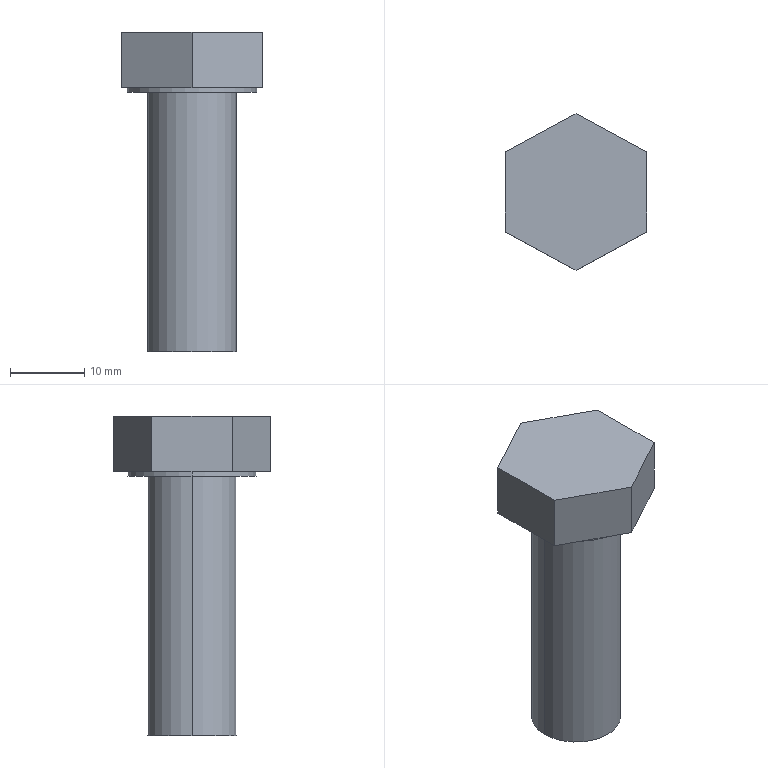Part | STEP file | M12-35 | 1 solid | 14 faces | box 19 x 21.1 x 43.1 mm | volume 6374 mm3 | plane 10 | cylinder 4 | commonest cylinder face diameters 12 x2 17.4 x2
STEP:
#1=CARTESIAN_POINT('',(0.,0.,0.));
#2=DIRECTION('',(0.,0.,1.));
#3=DIRECTION('',(1.,0.,0.));
#4=AXIS2_PLACEMENT_3D('',#1,#2,#3);
#5=CARTESIAN_POINT('',(0.,10.55,0.));
#6=VERTEX_POINT('',#5);
#7=CARTESIAN_POINT('',(-9.5,5.402,0.));
#8=VERTEX_POINT('',#7);
#9=CARTESIAN_POINT('',(0.,10.55,0.));
#10=DIRECTION('',(-0.8792,-0.4764,0.));
#11=VECTOR('',#10,1.);
#12=LINE('',#9,#11);
#13=CARTESIAN_POINT('',(0.,0.,0.));
#14=DIRECTION('',(0.,0.,1.));
#15=DIRECTION('',(1.,0.,0.));
#16=AXIS2_PLACEMENT_3D('',#13,#14,#15);
#17=PLANE('',#16);
#18=CARTESIAN_POINT('',(0.,10.55));
#19=DIRECTION('',(-0.8792,-0.4764));
#20=VECTOR('',#19,1.);
#21=LINE('',#18,#20);
#22=(GEOMETRIC_REPRESENTATION_CONTEXT(2)PARAMETRIC_REPRESENTATION_CONTEXT()REPRESENTATION_CONTEXT('',''));
#23=DEFINITIONAL_REPRESENTATION('',(#21),#22);
#24=PCURVE('',#17,#23);
#25=CARTESIAN_POINT('',(0.,10.55,0.));
#26=DIRECTION('',(-0.4764,0.8792,0.));
#27=DIRECTION('',(-0.8792,-0.4764,0.));
#28=AXIS2_PLACEMENT_3D('',#25,#26,#27);
#29=PLANE('',#28);
#30=CARTESIAN_POINT('',(0.,0.));
#31=DIRECTION('',(1.,0.));
#32=VECTOR('',#31,1.);
#33=LINE('',#30,#32);
#34=(GEOMETRIC_REPRESENTATION_CONTEXT(2)PARAMETRIC_REPRESENTATION_CONTEXT()REPRESENTATION_CONTEXT('',''));
#35=DEFINITIONAL_REPRESENTATION('',(#33),#34);
#36=PCURVE('',#29,#35);
#37=SURFACE_CURVE('',#12,(#24,#36),.PCURVE_S1.);
#38=EDGE_CURVE('',#6,#8,#37,.T.);
#39=ORIENTED_EDGE('',*,*,#38,.T.);
#40=CARTESIAN_POINT('',(-9.5,-5.402,0.));
#41=VERTEX_POINT('',#40);
#42=CARTESIAN_POINT('',(-9.5,5.402,0.));
#43=DIRECTION('',(0.,-1.,0.));
#44=VECTOR('',#43,1.);
#45=LINE('',#42,#44);
#46=CARTESIAN_POINT('',(-9.5,5.402));
#47=DIRECTION('',(0.,-1.));
#48=VECTOR('',#47,1.);
#49=LINE('',#46,#48);
#50=(GEOMETRIC_REPRESENTATION_CONTEXT(2)PARAMETRIC_REPRESENTATION_CONTEXT()REPRESENTATION_CONTEXT('',''));
#51=DEFINITIONAL_REPRESENTATION('',(#49),#50);
#52=PCURVE('',#17,#51);
#53=CARTESIAN_POINT('',(-9.5,5.402,0.));
#54=DIRECTION('',(-1.,0.,0.));
#55=DIRECTION('',(0.,-1.,0.));
#56=AXIS2_PLACEMENT_3D('',#53,#54,#55);
#57=PLANE('',#56);
#58=CARTESIAN_POINT('',(0.,0.));
#59=DIRECTION('',(1.,0.));
#60=VECTOR('',#59,1.);
#61=LINE('',#58,#60);
#62=(GEOMETRIC_REPRESENTATION_CONTEXT(2)PARAMETRIC_REPRESENTATION_CONTEXT()REPRESENTATION_CONTEXT('',''));
#63=DEFINITIONAL_REPRESENTATION('',(#61),#62);
#64=PCURVE('',#57,#63);
#65=SURFACE_CURVE('',#45,(#52,#64),.PCURVE_S1.);
#66=EDGE_CURVE('',#8,#41,#65,.T.);
#67=ORIENTED_EDGE('',*,*,#66,.T.);
#68=CARTESIAN_POINT('',(0.,-10.55,0.));
#69=VERTEX_POINT('',#68);
#70=CARTESIAN_POINT('',(-9.5,-5.402,0.));
#71=DIRECTION('',(0.8792,-0.4764,0.));
#72=VECTOR('',#71,1.);
#73=LINE('',#70,#72);
#74=CARTESIAN_POINT('',(-9.5,-5.402));
#75=DIRECTION('',(0.8792,-0.4764));
#76=VECTOR('',#75,1.);
#77=LINE('',#74,#76);
#78=(GEOMETRIC_REPRESENTATION_CONTEXT(2)PARAMETRIC_REPRESENTATION_CONTEXT()REPRESENTATION_CONTEXT('',''));
#79=DEFINITIONAL_REPRESENTATION('',(#77),#78);
#80=PCURVE('',#17,#79);
#81=CARTESIAN_POINT('',(-9.5,-5.402,0.));
#82=DIRECTION('',(-0.4764,-0.8792,0.));
#83=DIRECTION('',(0.8792,-0.4764,0.));
#84=AXIS2_PLACEMENT_3D('',#81,#82,#83);
#85=PLANE('',#84);
#86=CARTESIAN_POINT('',(0.,0.));
#87=DIRECTION('',(1.,0.));
#88=VECTOR('',#87,1.);
#89=LINE('',#86,#88);
#90=(GEOMETRIC_REPRESENTATION_CONTEXT(2)PARAMETRIC_REPRESENTATION_CONTEXT()REPRESENTATION_CONTEXT('',''));
#91=DEFINITIONAL_REPRESENTATION('',(#89),#90);
#92=PCURVE('',#85,#91);
#93=SURFACE_CURVE('',#73,(#80,#92),.PCURVE_S1.);
#94=EDGE_CURVE('',#41,#69,#93,.T.);
#95=ORIENTED_EDGE('',*,*,#94,.T.);
#96=CARTESIAN_POINT('',(9.5,-5.402,0.));
#97=VERTEX_POINT('',#96);
#98=CARTESIAN_POINT('',(0.,-10.55,0.));
#99=DIRECTION('',(0.8792,0.4764,0.));
#100=VECTOR('',#99,1.);
#101=LINE('',#98,#100);
#102=CARTESIAN_POINT('',(0.,-10.55));
#103=DIRECTION('',(0.8792,0.4764));
#104=VECTOR('',#103,1.);
#105=LINE('',#102,#104);
#106=(GEOMETRIC_REPRESENTATION_CONTEXT(2)PARAMETRIC_REPRESENTATION_CONTEXT()REPRESENTATION_CONTEXT('',''));
#107=DEFINITIONAL_REPRESENTATION('',(#105),#106);
#108=PCURVE('',#17,#107);
#109=CARTESIAN_POINT('',(0.,-10.55,0.));
#110=DIRECTION('',(0.4764,-0.8792,0.));
#111=DIRECTION('',(0.8792,0.4764,0.));
#112=AXIS2_PLACEMENT_3D('',#109,#110,#111);
#113=PLANE('',#112);
#114=CARTESIAN_POINT('',(0.,0.));
#115=DIRECTION('',(1.,0.));
#116=VECTOR('',#115,1.);
#117=LINE('',#114,#116);
#118=(GEOMETRIC_REPRESENTATION_CONTEXT(2)PARAMETRIC_REPRESENTATION_CONTEXT()REPRESENTATION_CONTEXT('',''));
#119=DEFINITIONAL_REPRESENTATION('',(#117),#118);
#120=PCURVE('',#113,#119);
#121=SURFACE_CURVE('',#101,(#108,#120),.PCURVE_S1.);
#122=EDGE_CURVE('',#69,#97,#121,.T.);
#123=ORIENTED_EDGE('',*,*,#122,.T.);
#124=CARTESIAN_POINT('',(9.5,5.402,0.));
#125=VERTEX_POINT('',#124);
#126=CARTESIAN_POINT('',(9.5,-5.402,0.));
#127=DIRECTION('',(0.,1.,0.));
#128=VECTOR('',#127,1.);
#129=LINE('',#126,#128);
#130=CARTESIAN_POINT('',(9.5,-5.402));
#131=DIRECTION('',(0.,1.));
#132=VECTOR('',#131,1.);
#133=LINE('',#130,#132);
#134=(GEOMETRIC_REPRESENTATION_CONTEXT(2)PARAMETRIC_REPRESENTATION_CONTEXT()REPRESENTATION_CONTEXT('',''));
#135=DEFINITIONAL_REPRESENTATION('',(#133),#134);
#136=PCURVE('',#17,#135);
#137=CARTESIAN_POINT('',(9.5,-5.402,0.));
#138=DIRECTION('',(1.,0.,0.));
#139=DIRECTION('',(0.,1.,0.));
#140=AXIS2_PLACEMENT_3D('',#137,#138,#139);
#141=PLANE('',#140);
#142=CARTESIAN_POINT('',(0.,0.));
#143=DIRECTION('',(1.,0.));
#144=VECTOR('',#143,1.);
#145=LINE('',#142,#144);
#146=(GEOMETRIC_REPRESENTATION_CONTEXT(2)PARAMETRIC_REPRESENTATION_CONTEXT()REPRESENTATION_CONTEXT('',''));
#147=DEFINITIONAL_REPRESENTATION('',(#145),#146);
#148=PCURVE('',#141,#147);
#149=SURFACE_CURVE('',#129,(#136,#148),.PCURVE_S1.);
#150=EDGE_CURVE('',#97,#125,#149,.T.);
#151=ORIENTED_EDGE('',*,*,#150,.T.);
#152=CARTESIAN_POINT('',(9.5,5.402,0.));
#153=DIRECTION('',(-0.8792,0.4764,0.));
#154=VECTOR('',#153,1.);
#155=LINE('',#152,#154);
#156=CARTESIAN_POINT('',(9.5,5.402));
#157=DIRECTION('',(-0.8792,0.4764));
#158=VECTOR('',#157,1.);
#159=LINE('',#156,#158);
#160=(GEOMETRIC_REPRESENTATION_CONTEXT(2)PARAMETRIC_REPRESENTATION_CONTEXT()REPRESENTATION_CONTEXT('',''));
#161=DEFINITIONAL_REPRESENTATION('',(#159),#160);
#162=PCURVE('',#17,#161);
#163=CARTESIAN_POINT('',(9.5,5.402,0.));
#164=DIRECTION('',(0.4764,0.8792,0.));
#165=DIRECTION('',(-0.8792,0.4764,0.));
#166=AXIS2_PLACEMENT_3D('',#163,#164,#165);
#167=PLANE('',#166);
#168=CARTESIAN_POINT('',(0.,0.));
#169=DIRECTION('',(1.,0.));
#170=VECTOR('',#169,1.);
#171=LINE('',#168,#170);
#172=(GEOMETRIC_REPRESENTATION_CONTEXT(2)PARAMETRIC_REPRESENTATION_CONTEXT()REPRESENTATION_CONTEXT('',''));
#173=DEFINITIONAL_REPRESENTATION('',(#171),#172);
#174=PCURVE('',#167,#173);
#175=SURFACE_CURVE('',#155,(#162,#174),.PCURVE_S1.);
#176=EDGE_CURVE('',#125,#6,#175,.T.);
#177=ORIENTED_EDGE('',*,*,#176,.T.);
#178=EDGE_LOOP('',(#39,#67,#95,#123,#151,#177));
#179=FACE_BOUND('',#178,.F.);
#180=CARTESIAN_POINT('',(-8.7,0.,0.));
#181=VERTEX_POINT('',#180);
#182=CARTESIAN_POINT('',(8.7,0.,0.));
#183=VERTEX_POINT('',#182);
#184=CARTESIAN_POINT('',(0.,0.,0.));
#185=DIRECTION('',(0.,0.,-1.));
#186=DIRECTION('',(-1.,0.,0.));
#187=AXIS2_PLACEMENT_3D('',#184,#185,#186);
#188=CIRCLE('',#187,8.7);
#189=CARTESIAN_POINT('',(-8.7,0.));
#190=CARTESIAN_POINT('',(-8.7,15.069));
#191=CARTESIAN_POINT('',(4.35,7.534));
#192=CARTESIAN_POINT('',(17.4,0.));
#193=CARTESIAN_POINT('',(4.35,-7.534));
#194=CARTESIAN_POINT('',(-8.7,-15.069));
#195=CARTESIAN_POINT('',(-8.7,0.));
#196=(BOUNDED_CURVE()B_SPLINE_CURVE(2,(#189,#190,#191,#192,#193,#194,#195),.UNSPECIFIED.,.T.,.F.)B_SPLINE_CURVE_WITH_KNOTS((1,2,2,2,2,1),(-2.094,0.,2.094,4.189,6.283,8.378),.UNSPECIFIED.)CURVE()GEOMETRIC_REPRESENTATION_ITEM()RATIONAL_B_SPLINE_CURVE((1.,0.5,1.,0.5,1.,0.5,1.))REPRESENTATION_ITEM(''));
#197=(GEOMETRIC_REPRESENTATION_CONTEXT(2)PARAMETRIC_REPRESENTATION_CONTEXT()REPRESENTATION_CONTEXT('',''));
#198=DEFINITIONAL_REPRESENTATION('',(#196),#197);
#199=PCURVE('',#17,#198);
#200=CARTESIAN_POINT('',(0.,0.,0.));
#201=DIRECTION('',(0.,0.,-1.));
#202=DIRECTION('',(-1.,0.,0.));
#203=AXIS2_PLACEMENT_3D('',#200,#201,#202);
#204=CYLINDRICAL_SURFACE('',#203,8.7);
#205=CARTESIAN_POINT('',(0.,0.));
#206=DIRECTION('',(1.,0.));
#207=VECTOR('',#206,1.);
#208=LINE('',#205,#207);
#209=(GEOMETRIC_REPRESENTATION_CONTEXT(2)PARAMETRIC_REPRESENTATION_CONTEXT()REPRESENTATION_CONTEXT('',''));
#210=DEFINITIONAL_REPRESENTATION('',(#208),#209);
#211=PCURVE('',#204,#210);
#212=SURFACE_CURVE('',#188,(#199,#211),.PCURVE_S1.);
#213=EDGE_CURVE('',#181,#183,#212,.T.);
#214=ORIENTED_EDGE('',*,*,#213,.T.);
#215=CARTESIAN_POINT('',(0.,0.,0.));
#216=DIRECTION('',(0.,0.,-1.));
#217=DIRECTION('',(1.,0.,0.));
#218=AXIS2_PLACEMENT_3D('',#215,#216,#217);
#219=CIRCLE('',#218,8.7);
#220=CARTESIAN_POINT('',(8.7,0.));
#221=CARTESIAN_POINT('',(8.7,-15.069));
#222=CARTESIAN_POINT('',(-4.35,-7.534));
#223=CARTESIAN_POINT('',(-17.4,0.));
#224=CARTESIAN_POINT('',(-4.35,7.534));
#225=CARTESIAN_POINT('',(8.7,15.069));
#226=CARTESIAN_POINT('',(8.7,0.));
#227=(BOUNDED_CURVE()B_SPLINE_CURVE(2,(#220,#221,#222,#223,#224,#225,#226),.UNSPECIFIED.,.T.,.F.)B_SPLINE_CURVE_WITH_KNOTS((1,2,2,2,2,1),(-2.094,0.,2.094,4.189,6.283,8.378),.UNSPECIFIED.)CURVE()GEOMETRIC_REPRESENTATION_ITEM()RATIONAL_B_SPLINE_CURVE((1.,0.5,1.,0.5,1.,0.5,1.))REPRESENTATION_ITEM(''));
#228=(GEOMETRIC_REPRESENTATION_CONTEXT(2)PARAMETRIC_REPRESENTATION_CONTEXT()REPRESENTATION_CONTEXT('',''));
#229=DEFINITIONAL_REPRESENTATION('',(#227),#228);
#230=PCURVE('',#17,#229);
#231=CARTESIAN_POINT('',(0.,0.,0.));
#232=DIRECTION('',(0.,0.,-1.));
#233=DIRECTION('',(-1.,0.,0.));
#234=AXIS2_PLACEMENT_3D('',#231,#232,#233);
#235=CYLINDRICAL_SURFACE('',#234,8.7);
#236=CARTESIAN_POINT('',(3.142,0.));
#237=DIRECTION('',(1.,0.));
#238=VECTOR('',#237,1.);
#239=LINE('',#236,#238);
#240=(GEOMETRIC_REPRESENTATION_CONTEXT(2)PARAMETRIC_REPRESENTATION_CONTEXT()REPRESENTATION_CONTEXT('',''));
#241=DEFINITIONAL_REPRESENTATION('',(#239),#240);
#242=PCURVE('',#235,#241);
#243=SURFACE_CURVE('',#219,(#230,#242),.PCURVE_S1.);
#244=EDGE_CURVE('',#183,#181,#243,.T.);
#245=ORIENTED_EDGE('',*,*,#244,.T.);
#246=EDGE_LOOP('',(#214,#245));
#247=FACE_BOUND('',#246,.F.);
#248=ADVANCED_FACE('',(#179,#247),#17,.F.);
#249=ORIENTED_EDGE('',*,*,#38,.F.);
#250=CARTESIAN_POINT('',(0.,10.55,7.5));
#251=VERTEX_POINT('',#250);
#252=CARTESIAN_POINT('',(0.,10.55,0.));
#253=DIRECTION('',(0.,0.,1.));
#254=VECTOR('',#253,1.);
#255=LINE('',#252,#254);
#256=CARTESIAN_POINT('',(0.,0.));
#257=DIRECTION('',(0.,1.));
#258=VECTOR('',#257,1.);
#259=LINE('',#256,#258);
#260=(GEOMETRIC_REPRESENTATION_CONTEXT(2)PARAMETRIC_REPRESENTATION_CONTEXT()REPRESENTATION_CONTEXT('',''));
#261=DEFINITIONAL_REPRESENTATION('',(#259),#260);
#262=PCURVE('',#29,#261);
#263=CARTESIAN_POINT('',(10.805,0.));
#264=DIRECTION('',(0.,1.));
#265=VECTOR('',#264,1.);
#266=LINE('',#263,#265);
#267=(GEOMETRIC_REPRESENTATION_CONTEXT(2)PARAMETRIC_REPRESENTATION_CONTEXT()REPRESENTATION_CONTEXT('',''));
#268=DEFINITIONAL_REPRESENTATION('',(#266),#267);
#269=PCURVE('',#167,#268);
#270=SURFACE_CURVE('',#255,(#262,#269),.PCURVE_S1.);
#271=EDGE_CURVE('',#6,#251,#270,.T.);
#272=ORIENTED_EDGE('',*,*,#271,.T.);
#273=CARTESIAN_POINT('',(-9.5,5.402,7.5));
#274=VERTEX_POINT('',#273);
#275=CARTESIAN_POINT('',(0.,10.55,7.5));
#276=DIRECTION('',(-0.8792,-0.4764,0.));
#277=VECTOR('',#276,1.);
#278=LINE('',#275,#277);
#279=CARTESIAN_POINT('',(0.,7.5));
#280=DIRECTION('',(1.,0.));
#281=VECTOR('',#280,1.);
#282=LINE('',#279,#281);
#283=(GEOMETRIC_REPRESENTATION_CONTEXT(2)PARAMETRIC_REPRESENTATION_CONTEXT()REPRESENTATION_CONTEXT('',''));
#284=DEFINITIONAL_REPRESENTATION('',(#282),#283);
#285=PCURVE('',#29,#284);
#286=CARTESIAN_POINT('',(0.,0.,7.5));
#287=DIRECTION('',(0.,0.,1.));
#288=DIRECTION('',(1.,0.,0.));
#289=AXIS2_PLACEMENT_3D('',#286,#287,#288);
#290=PLANE('',#289);
#291=CARTESIAN_POINT('',(0.,10.55));
#292=DIRECTION('',(-0.8792,-0.4764));
#293=VECTOR('',#292,1.);
#294=LINE('',#291,#293);
#295=(GEOMETRIC_REPRESENTATION_CONTEXT(2)PARAMETRIC_REPRESENTATION_CONTEXT()REPRESENTATION_CONTEXT('',''));
#296=DEFINITIONAL_REPRESENTATION('',(#294),#295);
#297=PCURVE('',#290,#296);
#298=SURFACE_CURVE('',#278,(#285,#297),.PCURVE_S1.);
#299=EDGE_CURVE('',#251,#274,#298,.T.);
#300=ORIENTED_EDGE('',*,*,#299,.T.);
#301=CARTESIAN_POINT('',(-9.5,5.402,0.));
#302=DIRECTION('',(0.,0.,1.));
#303=VECTOR('',#302,1.);
#304=LINE('',#301,#303);
#305=CARTESIAN_POINT('',(10.805,0.));
#306=DIRECTION('',(0.,1.));
#307=VECTOR('',#306,1.);
#308=LINE('',#305,#307);
#309=(GEOMETRIC_REPRESENTATION_CONTEXT(2)PARAMETRIC_REPRESENTATION_CONTEXT()REPRESENTATION_CONTEXT('',''));
#310=DEFINITIONAL_REPRESENTATION('',(#308),#309);
#311=PCURVE('',#29,#310);
#312=CARTESIAN_POINT('',(0.,0.));
#313=DIRECTION('',(0.,1.));
#314=VECTOR('',#313,1.);
#315=LINE('',#312,#314);
#316=(GEOMETRIC_REPRESENTATION_CONTEXT(2)PARAMETRIC_REPRESENTATION_CONTEXT()REPRESENTATION_CONTEXT('',''));
#317=DEFINITIONAL_REPRESENTATION('',(#315),#316);
#318=PCURVE('',#57,#317);
#319=SURFACE_CURVE('',#304,(#311,#318),.PCURVE_S1.);
#320=EDGE_CURVE('',#8,#274,#319,.T.);
#321=ORIENTED_EDGE('',*,*,#320,.F.);
#322=EDGE_LOOP('',(#249,#272,#300,#321));
#323=FACE_BOUND('',#322,.F.);
#324=ADVANCED_FACE('',(#323),#29,.T.);
#325=ORIENTED_EDGE('',*,*,#176,.F.);
#326=CARTESIAN_POINT('',(9.5,5.402,7.5));
#327=VERTEX_POINT('',#326);
#328=CARTESIAN_POINT('',(9.5,5.402,0.));
#329=DIRECTION('',(0.,0.,1.));
#330=VECTOR('',#329,1.);
#331=LINE('',#328,#330);
#332=CARTESIAN_POINT('',(0.,0.));
#333=DIRECTION('',(0.,1.));
#334=VECTOR('',#333,1.);
#335=LINE('',#332,#334);
#336=(GEOMETRIC_REPRESENTATION_CONTEXT(2)PARAMETRIC_REPRESENTATION_CONTEXT()REPRESENTATION_CONTEXT('',''));
#337=DEFINITIONAL_REPRESENTATION('',(#335),#336);
#338=PCURVE('',#167,#337);
#339=CARTESIAN_POINT('',(10.805,0.));
#340=DIRECTION('',(0.,1.));
#341=VECTOR('',#340,1.);
#342=LINE('',#339,#341);
#343=(GEOMETRIC_REPRESENTATION_CONTEXT(2)PARAMETRIC_REPRESENTATION_CONTEXT()REPRESENTATION_CONTEXT('',''));
#344=DEFINITIONAL_REPRESENTATION('',(#342),#343);
#345=PCURVE('',#141,#344);
#346=SURFACE_CURVE('',#331,(#338,#345),.PCURVE_S1.);
#347=EDGE_CURVE('',#125,#327,#346,.T.);
#348=ORIENTED_EDGE('',*,*,#347,.T.);
#349=CARTESIAN_POINT('',(9.5,5.402,7.5));
#350=DIRECTION('',(-0.8792,0.4764,0.));
#351=VECTOR('',#350,1.);
#352=LINE('',#349,#351);
#353=CARTESIAN_POINT('',(0.,7.5));
#354=DIRECTION('',(1.,0.));
#355=VECTOR('',#354,1.);
#356=LINE('',#353,#355);
#357=(GEOMETRIC_REPRESENTATION_CONTEXT(2)PARAMETRIC_REPRESENTATION_CONTEXT()REPRESENTATION_CONTEXT('',''));
#358=DEFINITIONAL_REPRESENTATION('',(#356),#357);
#359=PCURVE('',#167,#358);
#360=CARTESIAN_POINT('',(9.5,5.402));
#361=DIRECTION('',(-0.8792,0.4764));
#362=VECTOR('',#361,1.);
#363=LINE('',#360,#362);
#364=(GEOMETRIC_REPRESENTATION_CONTEXT(2)PARAMETRIC_REPRESENTATION_CONTEXT()REPRESENTATION_CONTEXT('',''));
#365=DEFINITIONAL_REPRESENTATION('',(#363),#364);
#366=PCURVE('',#290,#365);
#367=SURFACE_CURVE('',#352,(#359,#366),.PCURVE_S1.);
#368=EDGE_CURVE('',#327,#251,#367,.T.);
#369=ORIENTED_EDGE('',*,*,#368,.T.);
#370=ORIENTED_EDGE('',*,*,#271,.F.);
#371=EDGE_LOOP('',(#325,#348,#369,#370));
#372=FACE_BOUND('',#371,.F.);
#373=ADVANCED_FACE('',(#372),#167,.T.);
#374=ORIENTED_EDGE('',*,*,#150,.F.);
#375=CARTESIAN_POINT('',(9.5,-5.402,7.5));
#376=VERTEX_POINT('',#375);
#377=CARTESIAN_POINT('',(9.5,-5.402,0.));
#378=DIRECTION('',(0.,0.,1.));
#379=VECTOR('',#378,1.);
#380=LINE('',#377,#379);
#381=CARTESIAN_POINT('',(0.,0.));
#382=DIRECTION('',(0.,1.));
#383=VECTOR('',#382,1.);
#384=LINE('',#381,#383);
#385=(GEOMETRIC_REPRESENTATION_CONTEXT(2)PARAMETRIC_REPRESENTATION_CONTEXT()REPRESENTATION_CONTEXT('',''));
#386=DEFINITIONAL_REPRESENTATION('',(#384),#385);
#387=PCURVE('',#141,#386);
#388=CARTESIAN_POINT('',(10.805,0.));
#389=DIRECTION('',(0.,1.));
#390=VECTOR('',#389,1.);
#391=LINE('',#388,#390);
#392=(GEOMETRIC_REPRESENTATION_CONTEXT(2)PARAMETRIC_REPRESENTATION_CONTEXT()REPRESENTATION_CONTEXT('',''));
#393=DEFINITIONAL_REPRESENTATION('',(#391),#392);
#394=PCURVE('',#113,#393);
#395=SURFACE_CURVE('',#380,(#387,#394),.PCURVE_S1.);
#396=EDGE_CURVE('',#97,#376,#395,.T.);
#397=ORIENTED_EDGE('',*,*,#396,.T.);
#398=CARTESIAN_POINT('',(9.5,-5.402,7.5));
#399=DIRECTION('',(0.,1.,0.));
#400=VECTOR('',#399,1.);
#401=LINE('',#398,#400);
#402=CARTESIAN_POINT('',(0.,7.5));
#403=DIRECTION('',(1.,0.));
#404=VECTOR('',#403,1.);
#405=LINE('',#402,#404);
#406=(GEOMETRIC_REPRESENTATION_CONTEXT(2)PARAMETRIC_REPRESENTATION_CONTEXT()REPRESENTATION_CONTEXT('',''));
#407=DEFINITIONAL_REPRESENTATION('',(#405),#406);
#408=PCURVE('',#141,#407);
#409=CARTESIAN_POINT('',(9.5,-5.402));
#410=DIRECTION('',(0.,1.));
#411=VECTOR('',#410,1.);
#412=LINE('',#409,#411);
#413=(GEOMETRIC_REPRESENTATION_CONTEXT(2)PARAMETRIC_REPRESENTATION_CONTEXT()REPRESENTATION_CONTEXT('',''));
#414=DEFINITIONAL_REPRESENTATION('',(#412),#413);
#415=PCURVE('',#290,#414);
#416=SURFACE_CURVE('',#401,(#408,#415),.PCURVE_S1.);
#417=EDGE_CURVE('',#376,#327,#416,.T.);
#418=ORIENTED_EDGE('',*,*,#417,.T.);
#419=ORIENTED_EDGE('',*,*,#347,.F.);
#420=EDGE_LOOP('',(#374,#397,#418,#419));
#421=FACE_BOUND('',#420,.F.);
#422=ADVANCED_FACE('',(#421),#141,.T.);
#423=ORIENTED_EDGE('',*,*,#122,.F.);
#424=CARTESIAN_POINT('',(0.,-10.55,7.5));
#425=VERTEX_POINT('',#424);
#426=CARTESIAN_POINT('',(0.,-10.55,0.));
#427=DIRECTION('',(0.,0.,1.));
#428=VECTOR('',#427,1.);
#429=LINE('',#426,#428);
#430=CARTESIAN_POINT('',(0.,0.));
#431=DIRECTION('',(0.,1.));
#432=VECTOR('',#431,1.);
#433=LINE('',#430,#432);
#434=(GEOMETRIC_REPRESENTATION_CONTEXT(2)PARAMETRIC_REPRESENTATION_CONTEXT()REPRESENTATION_CONTEXT('',''));
#435=DEFINITIONAL_REPRESENTATION('',(#433),#434);
#436=PCURVE('',#113,#435);
#437=CARTESIAN_POINT('',(10.805,0.));
#438=DIRECTION('',(0.,1.));
#439=VECTOR('',#438,1.);
#440=LINE('',#437,#439);
#441=(GEOMETRIC_REPRESENTATION_CONTEXT(2)PARAMETRIC_REPRESENTATION_CONTEXT()REPRESENTATION_CONTEXT('',''));
#442=DEFINITIONAL_REPRESENTATION('',(#440),#441);
#443=PCURVE('',#85,#442);
#444=SURFACE_CURVE('',#429,(#436,#443),.PCURVE_S1.);
#445=EDGE_CURVE('',#69,#425,#444,.T.);
#446=ORIENTED_EDGE('',*,*,#445,.T.);
#447=CARTESIAN_POINT('',(0.,-10.55,7.5));
#448=DIRECTION('',(0.8792,0.4764,0.));
#449=VECTOR('',#448,1.);
#450=LINE('',#447,#449);
#451=CARTESIAN_POINT('',(0.,7.5));
#452=DIRECTION('',(1.,0.));
#453=VECTOR('',#452,1.);
#454=LINE('',#451,#453);
#455=(GEOMETRIC_REPRESENTATION_CONTEXT(2)PARAMETRIC_REPRESENTATION_CONTEXT()REPRESENTATION_CONTEXT('',''));
#456=DEFINITIONAL_REPRESENTATION('',(#454),#455);
#457=PCURVE('',#113,#456);
#458=CARTESIAN_POINT('',(0.,-10.55));
#459=DIRECTION('',(0.8792,0.4764));
#460=VECTOR('',#459,1.);
#461=LINE('',#458,#460);
#462=(GEOMETRIC_REPRESENTATION_CONTEXT(2)PARAMETRIC_REPRESENTATION_CONTEXT()REPRESENTATION_CONTEXT('',''));
#463=DEFINITIONAL_REPRESENTATION('',(#461),#462);
#464=PCURVE('',#290,#463);
#465=SURFACE_CURVE('',#450,(#457,#464),.PCURVE_S1.);
#466=EDGE_CURVE('',#425,#376,#465,.T.);
#467=ORIENTED_EDGE('',*,*,#466,.T.);
#468=ORIENTED_EDGE('',*,*,#396,.F.);
#469=EDGE_LOOP('',(#423,#446,#467,#468));
#470=FACE_BOUND('',#469,.F.);
#471=ADVANCED_FACE('',(#470),#113,.T.);
#472=ORIENTED_EDGE('',*,*,#94,.F.);
#473=CARTESIAN_POINT('',(-9.5,-5.402,7.5));
#474=VERTEX_POINT('',#473);
#475=CARTESIAN_POINT('',(-9.5,-5.402,0.));
#476=DIRECTION('',(0.,0.,1.));
#477=VECTOR('',#476,1.);
#478=LINE('',#475,#477);
#479=CARTESIAN_POINT('',(0.,0.));
#480=DIRECTION('',(0.,1.));
#481=VECTOR('',#480,1.);
#482=LINE('',#479,#481);
#483=(GEOMETRIC_REPRESENTATION_CONTEXT(2)PARAMETRIC_REPRESENTATION_CONTEXT()REPRESENTATION_CONTEXT('',''));
#484=DEFINITIONAL_REPRESENTATION('',(#482),#483);
#485=PCURVE('',#85,#484);
#486=CARTESIAN_POINT('',(10.805,0.));
#487=DIRECTION('',(0.,1.));
#488=VECTOR('',#487,1.);
#489=LINE('',#486,#488);
#490=(GEOMETRIC_REPRESENTATION_CONTEXT(2)PARAMETRIC_REPRESENTATION_CONTEXT()REPRESENTATION_CONTEXT('',''));
#491=DEFINITIONAL_REPRESENTATION('',(#489),#490);
#492=PCURVE('',#57,#491);
#493=SURFACE_CURVE('',#478,(#485,#492),.PCURVE_S1.);
#494=EDGE_CURVE('',#41,#474,#493,.T.);
#495=ORIENTED_EDGE('',*,*,#494,.T.);
#496=CARTESIAN_POINT('',(-9.5,-5.402,7.5));
#497=DIRECTION('',(0.8792,-0.4764,0.));
#498=VECTOR('',#497,1.);
#499=LINE('',#496,#498);
#500=CARTESIAN_POINT('',(0.,7.5));
#501=DIRECTION('',(1.,0.));
#502=VECTOR('',#501,1.);
#503=LINE('',#500,#502);
#504=(GEOMETRIC_REPRESENTATION_CONTEXT(2)PARAMETRIC_REPRESENTATION_CONTEXT()REPRESENTATION_CONTEXT('',''));
#505=DEFINITIONAL_REPRESENTATION('',(#503),#504);
#506=PCURVE('',#85,#505);
#507=CARTESIAN_POINT('',(-9.5,-5.402));
#508=DIRECTION('',(0.8792,-0.4764));
#509=VECTOR('',#508,1.);
#510=LINE('',#507,#509);
#511=(GEOMETRIC_REPRESENTATION_CONTEXT(2)PARAMETRIC_REPRESENTATION_CONTEXT()REPRESENTATION_CONTEXT('',''));
#512=DEFINITIONAL_REPRESENTATION('',(#510),#511);
#513=PCURVE('',#290,#512);
#514=SURFACE_CURVE('',#499,(#506,#513),.PCURVE_S1.);
#515=EDGE_CURVE('',#474,#425,#514,.T.);
#516=ORIENTED_EDGE('',*,*,#515,.T.);
#517=ORIENTED_EDGE('',*,*,#445,.F.);
#518=EDGE_LOOP('',(#472,#495,#516,#517));
#519=FACE_BOUND('',#518,.F.);
#520=ADVANCED_FACE('',(#519),#85,.T.);
#521=ORIENTED_EDGE('',*,*,#66,.F.);
#522=ORIENTED_EDGE('',*,*,#320,.T.);
#523=CARTESIAN_POINT('',(-9.5,5.402,7.5));
#524=DIRECTION('',(0.,-1.,0.));
#525=VECTOR('',#524,1.);
#526=LINE('',#523,#525);
#527=CARTESIAN_POINT('',(0.,7.5));
#528=DIRECTION('',(1.,0.));
#529=VECTOR('',#528,1.);
#530=LINE('',#527,#529);
#531=(GEOMETRIC_REPRESENTATION_CONTEXT(2)PARAMETRIC_REPRESENTATION_CONTEXT()REPRESENTATION_CONTEXT('',''));
#532=DEFINITIONAL_REPRESENTATION('',(#530),#531);
#533=PCURVE('',#57,#532);
#534=CARTESIAN_POINT('',(-9.5,5.402));
#535=DIRECTION('',(0.,-1.));
#536=VECTOR('',#535,1.);
#537=LINE('',#534,#536);
#538=(GEOMETRIC_REPRESENTATION_CONTEXT(2)PARAMETRIC_REPRESENTATION_CONTEXT()REPRESENTATION_CONTEXT('',''));
#539=DEFINITIONAL_REPRESENTATION('',(#537),#538);
#540=PCURVE('',#290,#539);
#541=SURFACE_CURVE('',#526,(#533,#540),.PCURVE_S1.);
#542=EDGE_CURVE('',#274,#474,#541,.T.);
#543=ORIENTED_EDGE('',*,*,#542,.T.);
#544=ORIENTED_EDGE('',*,*,#494,.F.);
#545=EDGE_LOOP('',(#521,#522,#543,#544));
#546=FACE_BOUND('',#545,.F.);
#547=ADVANCED_FACE('',(#546),#57,.T.);
#548=ORIENTED_EDGE('',*,*,#299,.F.);
#549=ORIENTED_EDGE('',*,*,#368,.F.);
#550=ORIENTED_EDGE('',*,*,#417,.F.);
#551=ORIENTED_EDGE('',*,*,#466,.F.);
#552=ORIENTED_EDGE('',*,*,#515,.F.);
#553=ORIENTED_EDGE('',*,*,#542,.F.);
#554=EDGE_LOOP('',(#548,#549,#550,#551,#552,#553));
#555=FACE_BOUND('',#554,.F.);
#556=ADVANCED_FACE('',(#555),#290,.T.);
#557=CARTESIAN_POINT('',(8.7,0.,-0.6));
#558=VERTEX_POINT('',#557);
#559=CARTESIAN_POINT('',(8.7,0.,0.));
#560=DIRECTION('',(0.,0.,-1.));
#561=VECTOR('',#560,1.);
#562=LINE('',#559,#561);
#563=CARTESIAN_POINT('',(3.142,0.));
#564=DIRECTION('',(0.,1.));
#565=VECTOR('',#564,1.);
#566=LINE('',#563,#565);
#567=(GEOMETRIC_REPRESENTATION_CONTEXT(2)PARAMETRIC_REPRESENTATION_CONTEXT()REPRESENTATION_CONTEXT('',''));
#568=DEFINITIONAL_REPRESENTATION('',(#566),#567);
#569=PCURVE('',#204,#568);
#570=CARTESIAN_POINT('',(3.142,0.));
#571=DIRECTION('',(0.,1.));
#572=VECTOR('',#571,1.);
#573=LINE('',#570,#572);
#574=(GEOMETRIC_REPRESENTATION_CONTEXT(2)PARAMETRIC_REPRESENTATION_CONTEXT()REPRESENTATION_CONTEXT('',''));
#575=DEFINITIONAL_REPRESENTATION('',(#573),#574);
#576=PCURVE('',#235,#575);
#577=SURFACE_CURVE('',#562,(#569,#576),.PCURVE_S1.);
#578=EDGE_CURVE('',#183,#558,#577,.T.);
#579=ORIENTED_EDGE('',*,*,#578,.T.);
#580=CARTESIAN_POINT('',(-8.7,0.,-0.6));
#581=VERTEX_POINT('',#580);
#582=CARTESIAN_POINT('',(0.,0.,-0.6));
#583=DIRECTION('',(0.,0.,-1.));
#584=DIRECTION('',(-1.,0.,0.));
#585=AXIS2_PLACEMENT_3D('',#582,#583,#584);
#586=CIRCLE('',#585,8.7);
#587=CARTESIAN_POINT('',(0.,0.6));
#588=DIRECTION('',(1.,0.));
#589=VECTOR('',#588,1.);
#590=LINE('',#587,#589);
#591=(GEOMETRIC_REPRESENTATION_CONTEXT(2)PARAMETRIC_REPRESENTATION_CONTEXT()REPRESENTATION_CONTEXT('',''));
#592=DEFINITIONAL_REPRESENTATION('',(#590),#591);
#593=PCURVE('',#204,#592);
#594=CARTESIAN_POINT('',(0.,0.,-0.6));
#595=DIRECTION('',(0.,0.,-1.));
#596=DIRECTION('',(-1.,0.,0.));
#597=AXIS2_PLACEMENT_3D('',#594,#595,#596);
#598=PLANE('',#597);
#599=CARTESIAN_POINT('',(0.,0.));
#600=DIRECTION('',(1.,0.));
#601=AXIS2_PLACEMENT_2D('',#599,#600);
#602=CIRCLE('',#601,8.7);
#603=(GEOMETRIC_REPRESENTATION_CONTEXT(2)PARAMETRIC_REPRESENTATION_CONTEXT()REPRESENTATION_CONTEXT('',''));
#604=DEFINITIONAL_REPRESENTATION('',(#602),#603);
#605=PCURVE('',#598,#604);
#606=SURFACE_CURVE('',#586,(#593,#605),.PCURVE_S1.);
#607=EDGE_CURVE('',#581,#558,#606,.T.);
#608=ORIENTED_EDGE('',*,*,#607,.F.);
#609=CARTESIAN_POINT('',(-8.7,0.,0.));
#610=DIRECTION('',(0.,0.,-1.));
#611=VECTOR('',#610,1.);
#612=LINE('',#609,#611);
#613=CARTESIAN_POINT('',(0.,0.));
#614=DIRECTION('',(0.,1.));
#615=VECTOR('',#614,1.);
#616=LINE('',#613,#615);
#617=(GEOMETRIC_REPRESENTATION_CONTEXT(2)PARAMETRIC_REPRESENTATION_CONTEXT()REPRESENTATION_CONTEXT('',''));
#618=DEFINITIONAL_REPRESENTATION('',(#616),#617);
#619=PCURVE('',#204,#618);
#620=CARTESIAN_POINT('',(6.283,0.));
#621=DIRECTION('',(0.,1.));
#622=VECTOR('',#621,1.);
#623=LINE('',#620,#622);
#624=(GEOMETRIC_REPRESENTATION_CONTEXT(2)PARAMETRIC_REPRESENTATION_CONTEXT()REPRESENTATION_CONTEXT('',''));
#625=DEFINITIONAL_REPRESENTATION('',(#623),#624);
#626=PCURVE('',#235,#625);
#627=SURFACE_CURVE('',#612,(#619,#626),.PCURVE_S1.);
#628=EDGE_CURVE('',#181,#581,#627,.T.);
#629=ORIENTED_EDGE('',*,*,#628,.F.);
#630=ORIENTED_EDGE('',*,*,#213,.T.);
#631=EDGE_LOOP('',(#579,#608,#629,#630));
#632=FACE_BOUND('',#631,.T.);
#633=ADVANCED_FACE('',(#632),#204,.T.);
#634=ORIENTED_EDGE('',*,*,#628,.T.);
#635=CARTESIAN_POINT('',(0.,0.,-0.6));
#636=DIRECTION('',(0.,0.,-1.));
#637=DIRECTION('',(1.,0.,0.));
#638=AXIS2_PLACEMENT_3D('',#635,#636,#637);
#639=CIRCLE('',#638,8.7);
#640=CARTESIAN_POINT('',(3.142,0.6));
#641=DIRECTION('',(1.,0.));
#642=VECTOR('',#641,1.);
#643=LINE('',#640,#642);
#644=(GEOMETRIC_REPRESENTATION_CONTEXT(2)PARAMETRIC_REPRESENTATION_CONTEXT()REPRESENTATION_CONTEXT('',''));
#645=DEFINITIONAL_REPRESENTATION('',(#643),#644);
#646=PCURVE('',#235,#645);
#647=CARTESIAN_POINT('',(0.,0.));
#648=DIRECTION('',(-1.,0.));
#649=AXIS2_PLACEMENT_2D('',#647,#648);
#650=CIRCLE('',#649,8.7);
#651=(GEOMETRIC_REPRESENTATION_CONTEXT(2)PARAMETRIC_REPRESENTATION_CONTEXT()REPRESENTATION_CONTEXT('',''));
#652=DEFINITIONAL_REPRESENTATION('',(#650),#651);
#653=PCURVE('',#598,#652);
#654=SURFACE_CURVE('',#639,(#646,#653),.PCURVE_S1.);
#655=EDGE_CURVE('',#558,#581,#654,.T.);
#656=ORIENTED_EDGE('',*,*,#655,.F.);
#657=ORIENTED_EDGE('',*,*,#578,.F.);
#658=ORIENTED_EDGE('',*,*,#244,.T.);
#659=EDGE_LOOP('',(#634,#656,#657,#658));
#660=FACE_BOUND('',#659,.T.);
#661=ADVANCED_FACE('',(#660),#235,.T.);
#662=ORIENTED_EDGE('',*,*,#607,.F.);
#663=ORIENTED_EDGE('',*,*,#655,.F.);
#664=EDGE_LOOP('',(#662,#663));
#665=FACE_BOUND('',#664,.F.);
#666=CARTESIAN_POINT('',(-6.,0.,-0.6));
#667=VERTEX_POINT('',#666);
#668=CARTESIAN_POINT('',(6.,0.,-0.6));
#669=VERTEX_POINT('',#668);
#670=CARTESIAN_POINT('',(0.,0.,-0.6));
#671=DIRECTION('',(0.,0.,-1.));
#672=DIRECTION('',(-1.,0.,0.));
#673=AXIS2_PLACEMENT_3D('',#670,#671,#672);
#674=CIRCLE('',#673,6.);
#675=CARTESIAN_POINT('',(0.,0.));
#676=DIRECTION('',(1.,0.));
#677=AXIS2_PLACEMENT_2D('',#675,#676);
#678=CIRCLE('',#677,6.);
#679=(GEOMETRIC_REPRESENTATION_CONTEXT(2)PARAMETRIC_REPRESENTATION_CONTEXT()REPRESENTATION_CONTEXT('',''));
#680=DEFINITIONAL_REPRESENTATION('',(#678),#679);
#681=PCURVE('',#598,#680);
#682=CARTESIAN_POINT('',(0.,0.,-0.6));
#683=DIRECTION('',(0.,0.,-1.));
#684=DIRECTION('',(-1.,0.,0.));
#685=AXIS2_PLACEMENT_3D('',#682,#683,#684);
#686=CYLINDRICAL_SURFACE('',#685,6.);
#687=CARTESIAN_POINT('',(0.,0.));
#688=DIRECTION('',(1.,0.));
#689=VECTOR('',#688,1.);
#690=LINE('',#687,#689);
#691=(GEOMETRIC_REPRESENTATION_CONTEXT(2)PARAMETRIC_REPRESENTATION_CONTEXT()REPRESENTATION_CONTEXT('',''));
#692=DEFINITIONAL_REPRESENTATION('',(#690),#691);
#693=PCURVE('',#686,#692);
#694=SURFACE_CURVE('',#674,(#681,#693),.PCURVE_S1.);
#695=EDGE_CURVE('',#667,#669,#694,.T.);
#696=ORIENTED_EDGE('',*,*,#695,.T.);
#697=CARTESIAN_POINT('',(0.,0.,-0.6));
#698=DIRECTION('',(0.,0.,-1.));
#699=DIRECTION('',(1.,0.,0.));
#700=AXIS2_PLACEMENT_3D('',#697,#698,#699);
#701=CIRCLE('',#700,6.);
#702=CARTESIAN_POINT('',(0.,0.));
#703=DIRECTION('',(-1.,0.));
#704=AXIS2_PLACEMENT_2D('',#702,#703);
#705=CIRCLE('',#704,6.);
#706=(GEOMETRIC_REPRESENTATION_CONTEXT(2)PARAMETRIC_REPRESENTATION_CONTEXT()REPRESENTATION_CONTEXT('',''));
#707=DEFINITIONAL_REPRESENTATION('',(#705),#706);
#708=PCURVE('',#598,#707);
#709=CARTESIAN_POINT('',(0.,0.,-0.6));
#710=DIRECTION('',(0.,0.,-1.));
#711=DIRECTION('',(-1.,0.,0.));
#712=AXIS2_PLACEMENT_3D('',#709,#710,#711);
#713=CYLINDRICAL_SURFACE('',#712,6.);
#714=CARTESIAN_POINT('',(3.142,0.));
#715=DIRECTION('',(1.,0.));
#716=VECTOR('',#715,1.);
#717=LINE('',#714,#716);
#718=(GEOMETRIC_REPRESENTATION_CONTEXT(2)PARAMETRIC_REPRESENTATION_CONTEXT()REPRESENTATION_CONTEXT('',''));
#719=DEFINITIONAL_REPRESENTATION('',(#717),#718);
#720=PCURVE('',#713,#719);
#721=SURFACE_CURVE('',#701,(#708,#720),.PCURVE_S1.);
#722=EDGE_CURVE('',#669,#667,#721,.T.);
#723=ORIENTED_EDGE('',*,*,#722,.T.);
#724=EDGE_LOOP('',(#696,#723));
#725=FACE_BOUND('',#724,.F.);
#726=ADVANCED_FACE('',(#665,#725),#598,.T.);
#727=CARTESIAN_POINT('',(6.,0.,-35.6));
#728=VERTEX_POINT('',#727);
#729=CARTESIAN_POINT('',(6.,0.,-0.6));
#730=DIRECTION('',(0.,0.,-1.));
#731=VECTOR('',#730,1.);
#732=LINE('',#729,#731);
#733=CARTESIAN_POINT('',(3.142,0.));
#734=DIRECTION('',(0.,1.));
#735=VECTOR('',#734,1.);
#736=LINE('',#733,#735);
#737=(GEOMETRIC_REPRESENTATION_CONTEXT(2)PARAMETRIC_REPRESENTATION_CONTEXT()REPRESENTATION_CONTEXT('',''));
#738=DEFINITIONAL_REPRESENTATION('',(#736),#737);
#739=PCURVE('',#686,#738);
#740=CARTESIAN_POINT('',(3.142,0.));
#741=DIRECTION('',(0.,1.));
#742=VECTOR('',#741,1.);
#743=LINE('',#740,#742);
#744=(GEOMETRIC_REPRESENTATION_CONTEXT(2)PARAMETRIC_REPRESENTATION_CONTEXT()REPRESENTATION_CONTEXT('',''));
#745=DEFINITIONAL_REPRESENTATION('',(#743),#744);
#746=PCURVE('',#713,#745);
#747=SURFACE_CURVE('',#732,(#739,#746),.PCURVE_S1.);
#748=EDGE_CURVE('',#669,#728,#747,.T.);
#749=ORIENTED_EDGE('',*,*,#748,.T.);
#750=CARTESIAN_POINT('',(-6.,0.,-35.6));
#751=VERTEX_POINT('',#750);
#752=CARTESIAN_POINT('',(0.,0.,-35.6));
#753=DIRECTION('',(0.,0.,-1.));
#754=DIRECTION('',(-1.,0.,0.));
#755=AXIS2_PLACEMENT_3D('',#752,#753,#754);
#756=CIRCLE('',#755,6.);
#757=CARTESIAN_POINT('',(0.,35.));
#758=DIRECTION('',(1.,0.));
#759=VECTOR('',#758,1.);
#760=LINE('',#757,#759);
#761=(GEOMETRIC_REPRESENTATION_CONTEXT(2)PARAMETRIC_REPRESENTATION_CONTEXT()REPRESENTATION_CONTEXT('',''));
#762=DEFINITIONAL_REPRESENTATION('',(#760),#761);
#763=PCURVE('',#686,#762);
#764=CARTESIAN_POINT('',(0.,0.,-35.6));
#765=DIRECTION('',(0.,0.,-1.));
#766=DIRECTION('',(-1.,0.,0.));
#767=AXIS2_PLACEMENT_3D('',#764,#765,#766);
#768=PLANE('',#767);
#769=CARTESIAN_POINT('',(0.,0.));
#770=DIRECTION('',(1.,0.));
#771=AXIS2_PLACEMENT_2D('',#769,#770);
#772=CIRCLE('',#771,6.);
#773=(GEOMETRIC_REPRESENTATION_CONTEXT(2)PARAMETRIC_REPRESENTATION_CONTEXT()REPRESENTATION_CONTEXT('',''));
#774=DEFINITIONAL_REPRESENTATION('',(#772),#773);
#775=PCURVE('',#768,#774);
#776=SURFACE_CURVE('',#756,(#763,#775),.PCURVE_S1.);
#777=EDGE_CURVE('',#751,#728,#776,.T.);
#778=ORIENTED_EDGE('',*,*,#777,.F.);
#779=CARTESIAN_POINT('',(-6.,0.,-0.6));
#780=DIRECTION('',(0.,0.,-1.));
#781=VECTOR('',#780,1.);
#782=LINE('',#779,#781);
#783=CARTESIAN_POINT('',(0.,0.));
#784=DIRECTION('',(0.,1.));
#785=VECTOR('',#784,1.);
#786=LINE('',#783,#785);
#787=(GEOMETRIC_REPRESENTATION_CONTEXT(2)PARAMETRIC_REPRESENTATION_CONTEXT()REPRESENTATION_CONTEXT('',''));
#788=DEFINITIONAL_REPRESENTATION('',(#786),#787);
#789=PCURVE('',#686,#788);
#790=CARTESIAN_POINT('',(6.283,0.));
#791=DIRECTION('',(0.,1.));
#792=VECTOR('',#791,1.);
#793=LINE('',#790,#792);
#794=(GEOMETRIC_REPRESENTATION_CONTEXT(2)PARAMETRIC_REPRESENTATION_CONTEXT()REPRESENTATION_CONTEXT('',''));
#795=DEFINITIONAL_REPRESENTATION('',(#793),#794);
#796=PCURVE('',#713,#795);
#797=SURFACE_CURVE('',#782,(#789,#796),.PCURVE_S1.);
#798=EDGE_CURVE('',#667,#751,#797,.T.);
#799=ORIENTED_EDGE('',*,*,#798,.F.);
#800=ORIENTED_EDGE('',*,*,#695,.T.);
#801=EDGE_LOOP('',(#749,#778,#799,#800));
#802=FACE_BOUND('',#801,.T.);
#803=ADVANCED_FACE('',(#802),#686,.T.);
#804=ORIENTED_EDGE('',*,*,#798,.T.);
#805=CARTESIAN_POINT('',(0.,0.,-35.6));
#806=DIRECTION('',(0.,0.,-1.));
#807=DIRECTION('',(1.,0.,0.));
#808=AXIS2_PLACEMENT_3D('',#805,#806,#807);
#809=CIRCLE('',#808,6.);
#810=CARTESIAN_POINT('',(3.142,35.));
#811=DIRECTION('',(1.,0.));
#812=VECTOR('',#811,1.);
#813=LINE('',#810,#812);
#814=(GEOMETRIC_REPRESENTATION_CONTEXT(2)PARAMETRIC_REPRESENTATION_CONTEXT()REPRESENTATION_CONTEXT('',''));
#815=DEFINITIONAL_REPRESENTATION('',(#813),#814);
#816=PCURVE('',#713,#815);
#817=CARTESIAN_POINT('',(0.,0.));
#818=DIRECTION('',(-1.,0.));
#819=AXIS2_PLACEMENT_2D('',#817,#818);
#820=CIRCLE('',#819,6.);
#821=(GEOMETRIC_REPRESENTATION_CONTEXT(2)PARAMETRIC_REPRESENTATION_CONTEXT()REPRESENTATION_CONTEXT('',''));
#822=DEFINITIONAL_REPRESENTATION('',(#820),#821);
#823=PCURVE('',#768,#822);
#824=SURFACE_CURVE('',#809,(#816,#823),.PCURVE_S1.);
#825=EDGE_CURVE('',#728,#751,#824,.T.);
#826=ORIENTED_EDGE('',*,*,#825,.F.);
#827=ORIENTED_EDGE('',*,*,#748,.F.);
#828=ORIENTED_EDGE('',*,*,#722,.T.);
#829=EDGE_LOOP('',(#804,#826,#827,#828));
#830=FACE_BOUND('',#829,.T.);
#831=ADVANCED_FACE('',(#830),#713,.T.);
#832=ORIENTED_EDGE('',*,*,#777,.F.);
#833=ORIENTED_EDGE('',*,*,#825,.F.);
#834=EDGE_LOOP('',(#832,#833));
#835=FACE_BOUND('',#834,.F.);
#836=ADVANCED_FACE('',(#835),#768,.T.);
#837=CLOSED_SHELL('',(#248,#324,#373,#422,#471,#520,#547,#556,#633,#661,#726,#803,#831,#836));
#838=MANIFOLD_SOLID_BREP('',#837);
#839=(LENGTH_UNIT()NAMED_UNIT(*)SI_UNIT(.MILLI.,.METRE.));
#840=UNCERTAINTY_MEASURE_WITH_UNIT(LENGTH_MEASURE(0.0000001),#839,'','');
#841=(NAMED_UNIT(*)PLANE_ANGLE_UNIT()SI_UNIT($,.RADIAN.));
#842=(NAMED_UNIT(*)SI_UNIT($,.STERADIAN.)SOLID_ANGLE_UNIT());
#843=(GEOMETRIC_REPRESENTATION_CONTEXT(3)GLOBAL_UNCERTAINTY_ASSIGNED_CONTEXT((#840))GLOBAL_UNIT_ASSIGNED_CONTEXT((#839,#841,#842))REPRESENTATION_CONTEXT('',''));
#844=ADVANCED_BREP_SHAPE_REPRESENTATION('',(#4,#838),#843);